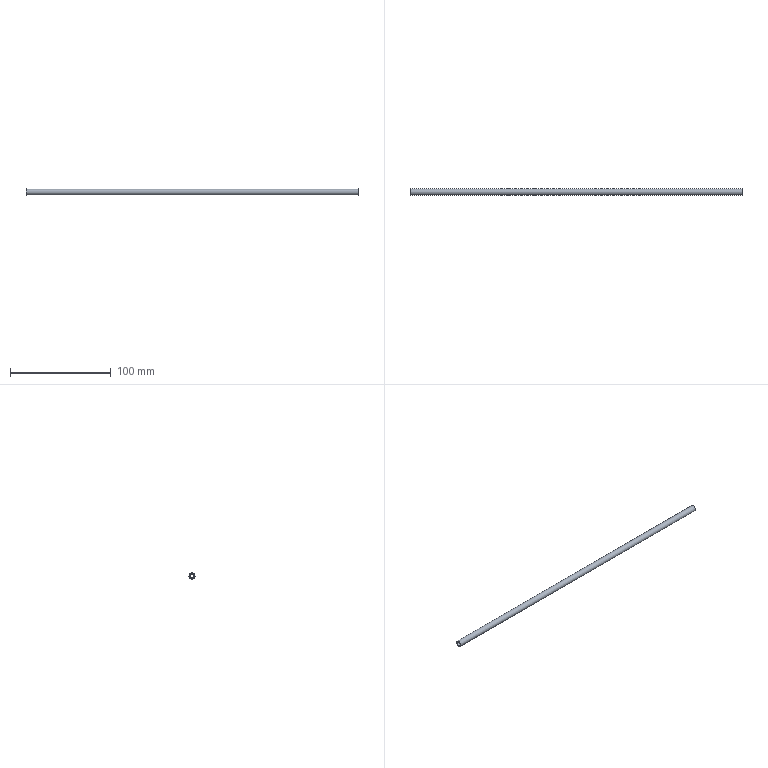Part | NX | features solid 2 | 1 solid | 4 faces | box 328.824 x 6 x 6 mm | volume 5165 mm3 | cylinder 2 | plane 2 | commonest cylinder face diameters 4 x1 6 x1
STEP:
#1=CARTESIAN_POINT('',(-423.824,-76.,347.));
#2=VERTEX_POINT('',#1);
#3=CARTESIAN_POINT('',(-423.824,-74.,347.));
#4=DIRECTION('',(-1.,0.,0.));
#5=DIRECTION('',(0.,-1.,0.));
#6=AXIS2_PLACEMENT_3D('',#3,#4,#5);
#7=CIRCLE('',#6,2.);
#8=EDGE_CURVE('',#2,#2,#7,.T.);
#9=ORIENTED_EDGE('',*,*,#8,.T.);
#10=EDGE_LOOP('',(#9));
#11=FACE_BOUND('',#10,.T.);
#12=CARTESIAN_POINT('',(-95.,-76.,347.));
#13=VERTEX_POINT('',#12);
#14=CARTESIAN_POINT('',(-95.,-74.,347.));
#15=DIRECTION('',(-1.,0.,0.));
#16=DIRECTION('',(0.,-1.,0.));
#17=AXIS2_PLACEMENT_3D('',#14,#15,#16);
#18=CIRCLE('',#17,2.);
#19=EDGE_CURVE('',#13,#13,#18,.T.);
#20=ORIENTED_EDGE('',*,*,#19,.F.);
#21=EDGE_LOOP('',(#20));
#22=FACE_BOUND('',#21,.T.);
#23=CARTESIAN_POINT('',(-273.824,-74.,347.));
#24=DIRECTION('',(1.,0.,0.));
#25=DIRECTION('',(0.,1.,0.));
#26=AXIS2_PLACEMENT_3D('',#23,#24,#25);
#27=CYLINDRICAL_SURFACE('',#26,2.);
#28=ADVANCED_FACE('',(#11,#22),#27,.F.);
#29=CARTESIAN_POINT('',(-423.824,-77.,347.));
#30=VERTEX_POINT('',#29);
#31=CARTESIAN_POINT('',(-423.824,-74.,347.));
#32=DIRECTION('',(-1.,0.,0.));
#33=DIRECTION('',(0.,-1.,0.));
#34=AXIS2_PLACEMENT_3D('',#31,#32,#33);
#35=CIRCLE('',#34,3.);
#36=EDGE_CURVE('',#30,#30,#35,.T.);
#37=ORIENTED_EDGE('',*,*,#36,.F.);
#38=EDGE_LOOP('',(#37));
#39=FACE_BOUND('',#38,.T.);
#40=CARTESIAN_POINT('',(-95.,-77.,347.));
#41=VERTEX_POINT('',#40);
#42=CARTESIAN_POINT('',(-95.,-74.,347.));
#43=DIRECTION('',(-1.,0.,0.));
#44=DIRECTION('',(0.,-1.,0.));
#45=AXIS2_PLACEMENT_3D('',#42,#43,#44);
#46=CIRCLE('',#45,3.);
#47=EDGE_CURVE('',#41,#41,#46,.T.);
#48=ORIENTED_EDGE('',*,*,#47,.T.);
#49=EDGE_LOOP('',(#48));
#50=FACE_BOUND('',#49,.T.);
#51=CARTESIAN_POINT('',(-273.824,-74.,347.));
#52=DIRECTION('',(1.,0.,0.));
#53=DIRECTION('',(0.,1.,0.));
#54=AXIS2_PLACEMENT_3D('',#51,#52,#53);
#55=CYLINDRICAL_SURFACE('',#54,3.);
#56=ADVANCED_FACE('',(#39,#50),#55,.T.);
#57=ORIENTED_EDGE('',*,*,#8,.F.);
#58=EDGE_LOOP('',(#57));
#59=FACE_BOUND('',#58,.T.);
#60=ORIENTED_EDGE('',*,*,#36,.T.);
#61=EDGE_LOOP('',(#60));
#62=FACE_BOUND('',#61,.T.);
#63=CARTESIAN_POINT('',(-423.824,-80.,347.));
#64=DIRECTION('',(-1.,0.,0.));
#65=DIRECTION('',(0.,-1.,0.));
#66=AXIS2_PLACEMENT_3D('',#63,#64,#65);
#67=PLANE('',#66);
#68=ADVANCED_FACE('',(#59,#62),#67,.T.);
#69=ORIENTED_EDGE('',*,*,#19,.T.);
#70=EDGE_LOOP('',(#69));
#71=FACE_BOUND('',#70,.T.);
#72=ORIENTED_EDGE('',*,*,#47,.F.);
#73=EDGE_LOOP('',(#72));
#74=FACE_BOUND('',#73,.T.);
#75=CARTESIAN_POINT('',(-95.,-74.,347.));
#76=DIRECTION('',(-1.,0.,0.));
#77=DIRECTION('',(0.,-1.,0.));
#78=AXIS2_PLACEMENT_3D('',#75,#76,#77);
#79=PLANE('',#78);
#80=ADVANCED_FACE('',(#71,#74),#79,.F.);
#81=CLOSED_SHELL('',(#28,#56,#68,#80));
#82=MANIFOLD_SOLID_BREP('',#81);
#83=(LENGTH_UNIT()NAMED_UNIT(*)SI_UNIT(.MILLI.,.METRE.));
#84=UNCERTAINTY_MEASURE_WITH_UNIT(LENGTH_MEASURE(0.00001),#83,'','');
#85=(NAMED_UNIT(*)PLANE_ANGLE_UNIT()SI_UNIT($,.RADIAN.));
#86=(NAMED_UNIT(*)SI_UNIT($,.STERADIAN.)SOLID_ANGLE_UNIT());
#87=(GEOMETRIC_REPRESENTATION_CONTEXT(3)GLOBAL_UNCERTAINTY_ASSIGNED_CONTEXT((#84))GLOBAL_UNIT_ASSIGNED_CONTEXT((#83,#85,#86))REPRESENTATION_CONTEXT('',''));
#88=ADVANCED_BREP_SHAPE_REPRESENTATION('',(#82),#87);